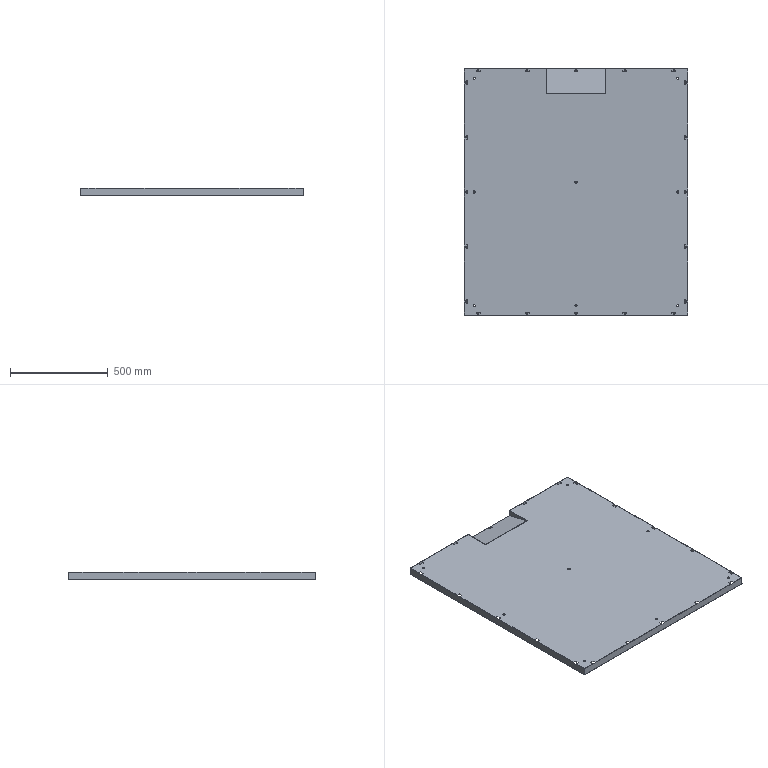Part | SolidWorks | 2 solids | 400 faces | box 1139 x 1259 x 40 mm | volume 1680362 mm3 | plane 254 | cylinder 126 | spline 20 | commonest cylinder face diameters 7 x50 0.4 x30 2.4 x30 11 x16